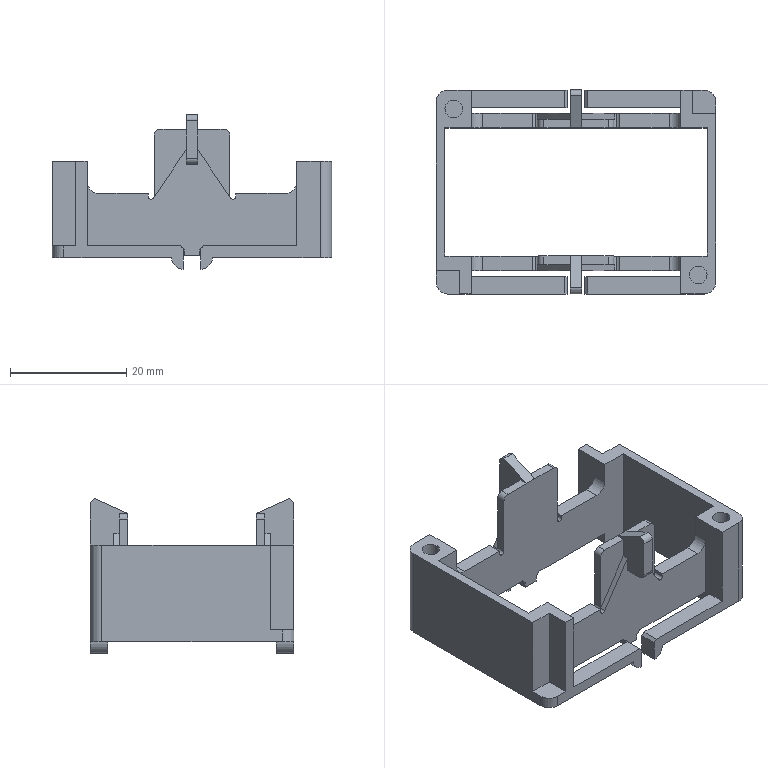Part | STEP file | Cover | 1 solid | 124 faces | box 48 x 35 x 26.5 mm | volume 5852 mm3 | plane 92 | cylinder 32 | commonest cylinder face diameters 4 x12 1 x8 2 x8 3 x4